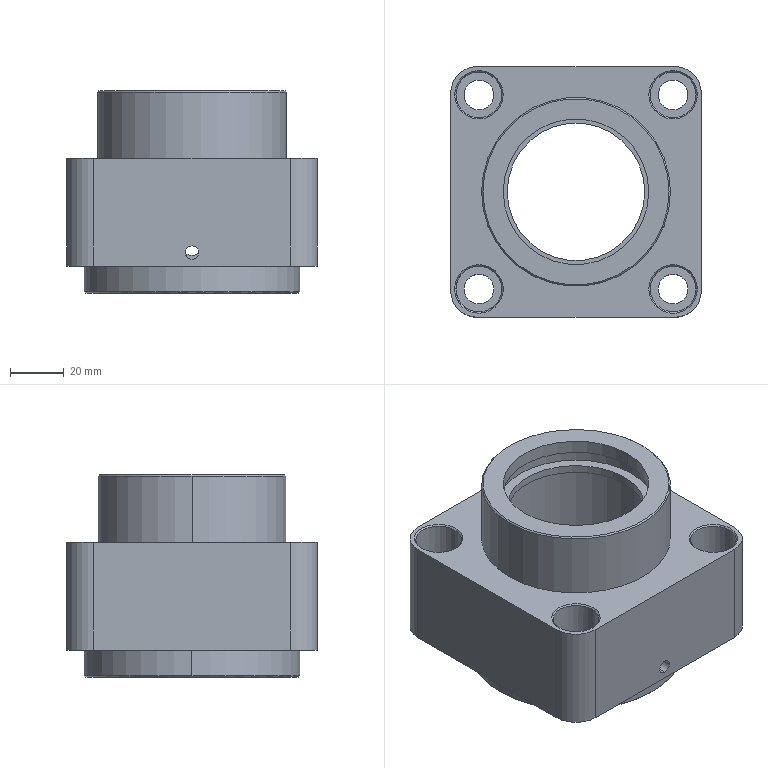Part | SolidWorks | features ICE 6, BaseBody 1, HoleWzd 1 | 1 solid | 78 faces | box 93 x 93 x 75 mm | volume 240309 mm3 | cylinder 44 | plane 18 | cone 16 | commonest cylinder face diameters 11 x8 17 x8 20 x4 60 x4 5 x2 8 x2